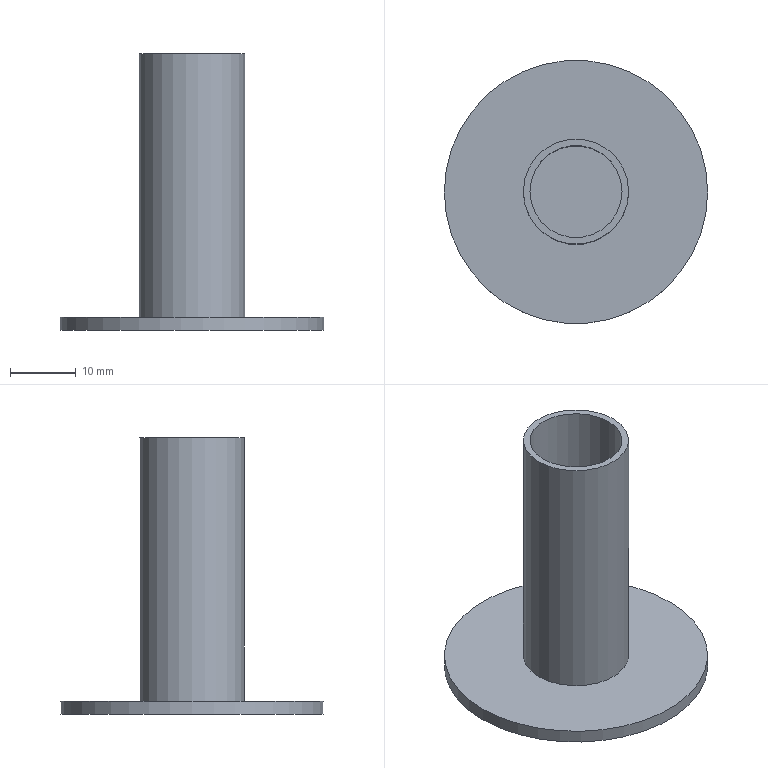Part | NX | features DATUM_CSYS 3, EXTRUDE 2, SKETCH 2 | 1 solid | 7 faces | box 40 x 40 x 42 mm | volume 4398 mm3 | plane 4 | cylinder 3 | commonest cylinder face diameters 14 x1 16 x1 40 x1
STEP:
#1=CARTESIAN_POINT('',(20.,0.,2.));
#2=VERTEX_POINT('',#1);
#3=CARTESIAN_POINT('',(0.,0.,2.));
#4=DIRECTION('',(0.,0.,1.));
#5=DIRECTION('',(1.,0.,0.));
#6=AXIS2_PLACEMENT_3D('',#3,#4,#5);
#7=CIRCLE('',#6,20.);
#8=EDGE_CURVE('',#2,#2,#7,.T.);
#9=ORIENTED_EDGE('',*,*,#8,.F.);
#10=EDGE_LOOP('',(#9));
#11=FACE_BOUND('',#10,.T.);
#12=CARTESIAN_POINT('',(20.,0.,0.));
#13=VERTEX_POINT('',#12);
#14=CARTESIAN_POINT('',(0.,0.,0.));
#15=DIRECTION('',(0.,0.,1.));
#16=DIRECTION('',(1.,0.,0.));
#17=AXIS2_PLACEMENT_3D('',#14,#15,#16);
#18=CIRCLE('',#17,20.);
#19=EDGE_CURVE('',#13,#13,#18,.T.);
#20=ORIENTED_EDGE('',*,*,#19,.T.);
#21=EDGE_LOOP('',(#20));
#22=FACE_BOUND('',#21,.T.);
#23=CARTESIAN_POINT('',(0.,0.,2.));
#24=DIRECTION('',(0.,0.,-1.));
#25=DIRECTION('',(-1.,0.,0.));
#26=AXIS2_PLACEMENT_3D('',#23,#24,#25);
#27=CYLINDRICAL_SURFACE('',#26,20.);
#28=ADVANCED_FACE('',(#11,#22),#27,.T.);
#29=CARTESIAN_POINT('',(8.,0.,2.));
#30=VERTEX_POINT('',#29);
#31=CARTESIAN_POINT('',(0.,0.,2.));
#32=DIRECTION('',(0.,0.,1.));
#33=DIRECTION('',(1.,0.,0.));
#34=AXIS2_PLACEMENT_3D('',#31,#32,#33);
#35=CIRCLE('',#34,8.);
#36=EDGE_CURVE('',#30,#30,#35,.T.);
#37=ORIENTED_EDGE('',*,*,#36,.F.);
#38=EDGE_LOOP('',(#37));
#39=FACE_BOUND('',#38,.T.);
#40=ORIENTED_EDGE('',*,*,#8,.T.);
#41=EDGE_LOOP('',(#40));
#42=FACE_BOUND('',#41,.T.);
#43=CARTESIAN_POINT('',(0.,0.,2.));
#44=DIRECTION('',(0.,0.,1.));
#45=DIRECTION('',(1.,0.,0.));
#46=AXIS2_PLACEMENT_3D('',#43,#44,#45);
#47=PLANE('',#46);
#48=ADVANCED_FACE('',(#39,#42),#47,.T.);
#49=ORIENTED_EDGE('',*,*,#19,.F.);
#50=EDGE_LOOP('',(#49));
#51=FACE_BOUND('',#50,.T.);
#52=CARTESIAN_POINT('',(0.,0.,0.));
#53=DIRECTION('',(0.,0.,1.));
#54=DIRECTION('',(1.,0.,0.));
#55=AXIS2_PLACEMENT_3D('',#52,#53,#54);
#56=PLANE('',#55);
#57=ADVANCED_FACE('',(#51),#56,.F.);
#58=CARTESIAN_POINT('',(8.,0.,42.));
#59=VERTEX_POINT('',#58);
#60=CARTESIAN_POINT('',(0.,0.,42.));
#61=DIRECTION('',(0.,0.,1.));
#62=DIRECTION('',(1.,0.,0.));
#63=AXIS2_PLACEMENT_3D('',#60,#61,#62);
#64=CIRCLE('',#63,8.);
#65=EDGE_CURVE('',#59,#59,#64,.T.);
#66=ORIENTED_EDGE('',*,*,#65,.F.);
#67=EDGE_LOOP('',(#66));
#68=FACE_BOUND('',#67,.T.);
#69=ORIENTED_EDGE('',*,*,#36,.T.);
#70=EDGE_LOOP('',(#69));
#71=FACE_BOUND('',#70,.T.);
#72=CARTESIAN_POINT('',(0.,0.,42.));
#73=DIRECTION('',(0.,0.,-1.));
#74=DIRECTION('',(-1.,0.,0.));
#75=AXIS2_PLACEMENT_3D('',#72,#73,#74);
#76=CYLINDRICAL_SURFACE('',#75,8.);
#77=ADVANCED_FACE('',(#68,#71),#76,.T.);
#78=CARTESIAN_POINT('',(7.,0.,42.));
#79=VERTEX_POINT('',#78);
#80=CARTESIAN_POINT('',(0.,0.,42.));
#81=DIRECTION('',(0.,0.,1.));
#82=DIRECTION('',(1.,0.,0.));
#83=AXIS2_PLACEMENT_3D('',#80,#81,#82);
#84=CIRCLE('',#83,7.);
#85=EDGE_CURVE('',#79,#79,#84,.T.);
#86=ORIENTED_EDGE('',*,*,#85,.T.);
#87=EDGE_LOOP('',(#86));
#88=FACE_BOUND('',#87,.T.);
#89=CARTESIAN_POINT('',(7.,0.,2.));
#90=VERTEX_POINT('',#89);
#91=CARTESIAN_POINT('',(0.,0.,2.));
#92=DIRECTION('',(0.,0.,1.));
#93=DIRECTION('',(1.,0.,0.));
#94=AXIS2_PLACEMENT_3D('',#91,#92,#93);
#95=CIRCLE('',#94,7.);
#96=EDGE_CURVE('',#90,#90,#95,.T.);
#97=ORIENTED_EDGE('',*,*,#96,.F.);
#98=EDGE_LOOP('',(#97));
#99=FACE_BOUND('',#98,.T.);
#100=CARTESIAN_POINT('',(0.,0.,42.));
#101=DIRECTION('',(0.,0.,-1.));
#102=DIRECTION('',(-1.,0.,0.));
#103=AXIS2_PLACEMENT_3D('',#100,#101,#102);
#104=CYLINDRICAL_SURFACE('',#103,7.);
#105=ADVANCED_FACE('',(#88,#99),#104,.F.);
#106=ORIENTED_EDGE('',*,*,#65,.T.);
#107=EDGE_LOOP('',(#106));
#108=FACE_BOUND('',#107,.T.);
#109=ORIENTED_EDGE('',*,*,#85,.F.);
#110=EDGE_LOOP('',(#109));
#111=FACE_BOUND('',#110,.T.);
#112=CARTESIAN_POINT('',(0.,0.,42.));
#113=DIRECTION('',(0.,0.,1.));
#114=DIRECTION('',(1.,0.,0.));
#115=AXIS2_PLACEMENT_3D('',#112,#113,#114);
#116=PLANE('',#115);
#117=ADVANCED_FACE('',(#108,#111),#116,.T.);
#118=ORIENTED_EDGE('',*,*,#96,.T.);
#119=EDGE_LOOP('',(#118));
#120=FACE_BOUND('',#119,.T.);
#121=CARTESIAN_POINT('',(0.,0.,2.));
#122=DIRECTION('',(0.,0.,1.));
#123=DIRECTION('',(1.,0.,0.));
#124=AXIS2_PLACEMENT_3D('',#121,#122,#123);
#125=PLANE('',#124);
#126=ADVANCED_FACE('',(#120),#125,.T.);
#127=CLOSED_SHELL('',(#28,#48,#57,#77,#105,#117,#126));
#128=MANIFOLD_SOLID_BREP('',#127);
#129=(LENGTH_UNIT()NAMED_UNIT(*)SI_UNIT(.MILLI.,.METRE.));
#130=UNCERTAINTY_MEASURE_WITH_UNIT(LENGTH_MEASURE(0.00001),#129,'','');
#131=(NAMED_UNIT(*)PLANE_ANGLE_UNIT()SI_UNIT($,.RADIAN.));
#132=(NAMED_UNIT(*)SI_UNIT($,.STERADIAN.)SOLID_ANGLE_UNIT());
#133=(GEOMETRIC_REPRESENTATION_CONTEXT(3)GLOBAL_UNCERTAINTY_ASSIGNED_CONTEXT((#130))GLOBAL_UNIT_ASSIGNED_CONTEXT((#129,#131,#132))REPRESENTATION_CONTEXT('',''));
#134=ADVANCED_BREP_SHAPE_REPRESENTATION('',(#128),#133);